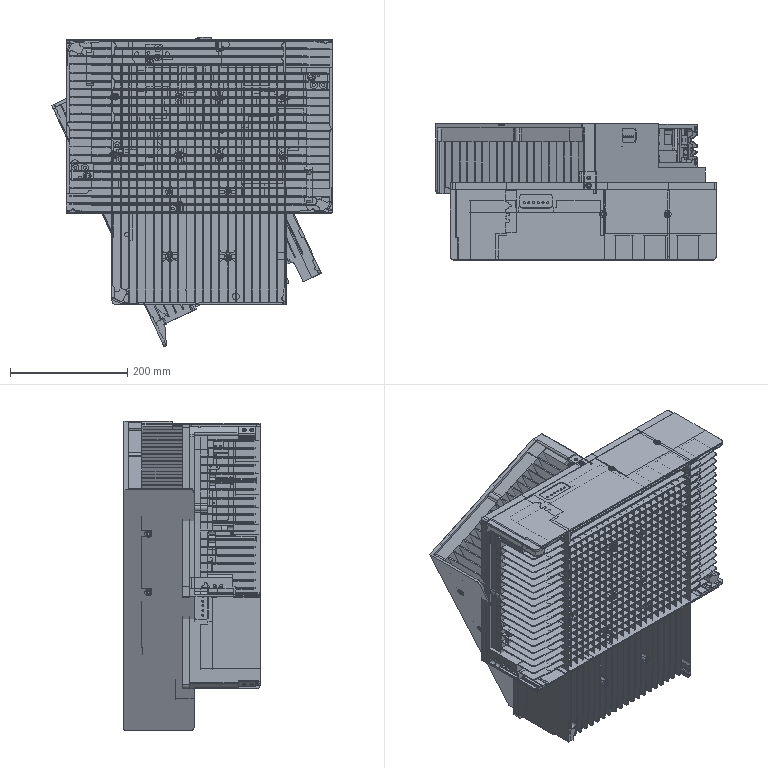NC program | NX | posted with a generic post
Whole program:
N10 G17 G21 G94 G90
(FACE_MILLING_COPY_COPY_COPY_1_COPY_3_COPY_COPY_1 , TOOL : D6_J)
N12 T04 M6
N14 G53
N16 G17 G0 G90 X70.882 Y-48.082 S8000 M3
N18 G43 Z20. H4
N20 Z-30.5
N22 G94 G1 X70.898 Y-48.098 Z-30.501 F1500.
N24 X72.83 Y-49.549 Z-30.628
N26 X74.935 Y-50.733 Z-30.754
N28 X77.177 Y-51.63 Z-30.881
N30 X78.191 Y-51.897 Z-30.936
N32 X77.177 Y-51.63 Z-30.991
N34 X74.935 Y-50.733 Z-31.117
N36 X72.83 Y-49.549 Z-31.244
N38 X70.898 Y-48.098 Z-31.371
N40 X69.175 Y-46.406 Z-31.497
N42 X67.689 Y-44.501 Z-31.624
N44 X67.15 Y-43.602 Z-31.679
N46 X67.689 Y-44.501 Z-31.734
N48 X69.175 Y-46.406 Z-31.86
N50 X70.898 Y-48.098 Z-31.987
N52 X72.83 Y-49.549 Z-32.113
N54 X74.935 Y-50.733 Z-32.24
N56 X77.177 Y-51.63 Z-32.367
N58 X78.191 Y-51.897 Z-32.422
N60 X77.177 Y-51.63 Z-32.476
N62 X74.935 Y-50.733 Z-32.603
N64 X72.83 Y-49.549 Z-32.73
N66 X70.898 Y-48.098 Z-32.856
N68 X69.175 Y-46.406 Z-32.983
N70 X67.689 Y-44.501 Z-33.109
N72 X67.15 Y-43.602 Z-33.164
N74 X67.689 Y-44.501 Z-33.219
N76 X69.175 Y-46.406 Z-33.346
N78 X70.898 Y-48.098 Z-33.472
N80 X72.83 Y-49.549 Z-33.599
N82 X74.935 Y-50.733 Z-33.726
N84 X77.177 Y-51.63 Z-33.852
N86 X78.191 Y-51.897 Z-33.907
N88 X77.177 Y-51.63 Z-33.962
N90 X74.935 Y-50.733 Z-34.089
N92 X72.83 Y-49.549 Z-34.215
N94 X70.898 Y-48.098 Z-34.342
N96 X69.175 Y-46.406 Z-34.468
N98 X67.689 Y-44.501 Z-34.595
N100 X67.15 Y-43.602 Z-34.65
N102 G3 X78.191 Y-51.897 R18.3
N104 X81.515 Y-47.332 R5.7
N106 G2 X69.65 Y-34.2 R13.2
N108 G1 Y-18.2
N110 G2 X73.384 Y-9. R13.2
N112 G1 Z-31.5
N114 G0 Z20.
N116 X81.515 Y-47.332
N118 Z-33.5
N120 G1 Z-34.65
N122 G3 X81.55 Y-46.7 R5.7
N124 G1 Y-43.4
N126 X126.85
N128 G3 X131.385 Y-41.153 R5.7
N130 G1 X127.982 Y-41.294
N132 G2 X126.316 Y-43.4 R13.2
N134 G1 Z-31.5
N136 G0 Z20.
N138 Z-33.5
N140 G1 Z-34.65
N142 X81.55
N144 Y-46.7
N146 G2 X75.85 Y-52.4 R5.7
N148 G1 X72.85
N150 G2 X67.15 Y-46.7 R5.7
N152 G1 Y-14.7
N154 G2 X72.85 Y-9. R5.7
N156 G1 X121.986
N158 Y-10.967
N160 G3 X122.051 Y-11.991 R8.1
N162 G1 X124.646 Y-13.497
N164 G3 X125.85 Y-15.216 R6.
N166 G1 Y-18.4
N168 Y-18.409
N170 X125.722 Y-18.444
N172 X124.218 Y-18.895
N174 G3 X123.02 Y-19.519 R3.6
N176 G1 X122.85 Y-19.653
N178 Y-18.2
N180 G3 X121.918 Y-14.988 R6.
N182 X124.646 Y-13.497 R3.
N184 G1 X122.051 Y-11.991
N186 G3 X116.85 Y-10.1 R8.1
N188 G1 X82.85
N190 G3 X74.75 Y-18.2 R8.1
N192 G1 Y-34.2
N194 G3 X82.85 Y-42.3 R8.1
N196 G1 X116.85
N198 G3 X124.777 Y-35.866 R8.1
N200 G1 X123.042 Y-33.16
N202 X124.777 Y-35.866
N204 X125.816 Y-36.177
N206 X128.215 Y-36.196
N208 X130.657 Y-36.082
N210 X132.55 Y-35.402
N212 Z-31.5
N214 G0 Z20.
N216 Z-33.5
N218 G1 Z-34.65
N220 Y-21.4
N222 X131.85
N224 G2 X128.85 Y-18.4 R3.
N226 G1 Y-13.7
N228 G2 X127.086 Y-10.967 R3.
N230 G1 Y-9.
N232 Z-31.5
N234 G0 Z20.
N236 X124.777 Y-35.866
N238 Z-31.5
N240 G1 Z-34.65
N242 X124.881 Y-30.529
N244 X124.534 Y-30.257
N246 G2 X124.38 Y-30.076 R0.6
N248 G1 X123.591 Y-28.655
N250 G2 X123.516 Y-28.385 R0.6
N252 G1 X123.467 Y-26.947
N254 Y-25.468
N256 X123.516 Y-24.03
N258 G2 X123.589 Y-23.763 R0.6
N260 G1 X124.363 Y-22.343
N262 G2 X124.518 Y-22.159 R0.6
N264 G1 X124.88 Y-21.873
N266 G2 X125.08 Y-21.769 R0.6
N268 G1 X126.584 Y-21.318
N270 X128.116 Y-21.306
N272 X129.652 Y-21.378
N274 X131.251 Y-21.944
N276 G2 X131.618 Y-22.314 R0.6
N278 G1 X132.173 Y-23.918
N280 X132.229 Y-25.467
N282 Y-26.949
N284 X132.176 Y-28.407
N286 X132.195 Y-28.506
N288 X132.14 Y-28.592
N290 X131.585 Y-30.101
N292 G2 X131.225 Y-30.459 R0.6
N294 G1 X129.653 Y-31.023
N296 X128.116 Y-31.095
N298 X126.584 Y-31.083
N300 X125.078 Y-30.632
N302 G2 X124.881 Y-30.529 R0.6
N304 G1 Z-31.5
N306 G0 Z20.
N308 X124.777 Y-35.866
N310 Z-33.5
N312 G1 Z-34.65
N314 X119.85 Y-34.2
N316 G2 X116.85 Y-37.2 R3.
N318 G1 X82.85
N320 G2 X79.85 Y-34.2 R3.
N322 G1 Y-18.2
N324 G2 X82.85 Y-15.2 R3.
N326 G1 X116.85
N328 G2 X119.85 Y-18.2 R3.
N330 G1 Y-34.2
N332 Z-31.5
N334 G0 Z20.
(PLANAR_PROFILE_COPY_COPY_COPY_COPY_COPY_COPY_COPY_COPY_COPY , TOOL : D6_J)
N336 X122.85 Y-27.2
N338 Z-33.5
N340 G1 Z-34.5
N342 G3 X123.85 Y-26.2 R1.
N344 G1 Y-24.7
N346 G2 X126.85 Y-21.7 R3.
N348 G1 X128.85
N350 G2 X131.85 Y-24.7 R3.
N352 G1 Y-27.7
N354 G2 X128.85 Y-30.7 R3.
N356 G1 X126.85
N358 G2 X123.85 Y-27.7 R3.
N360 G1 Y-26.2
N362 G3 X122.85 Y-25.2 R1.
N364 G1 Z-33.5
N366 G0 Z20.
N368 M5
N370 M2